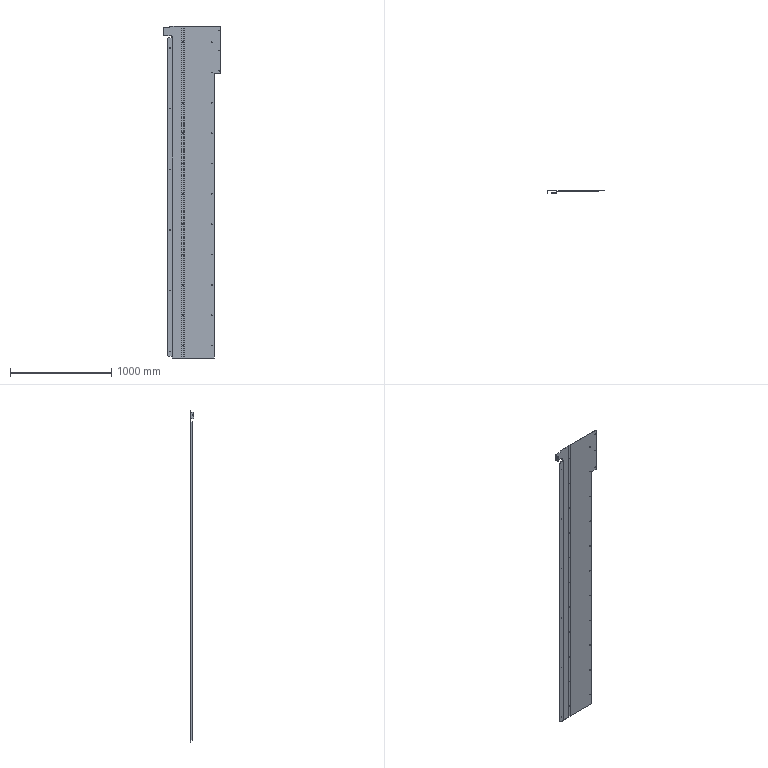Part | STEP file | TS-S34 | 1 solid | 148 faces | box 561 x 33 x 3283 mm | volume 1948503 mm3 | cylinder 86 | plane 62 | commonest cylinder face diameters 5.4 x64 0.4 x7 2.8 x7 10 x4 30 x2 22 x1